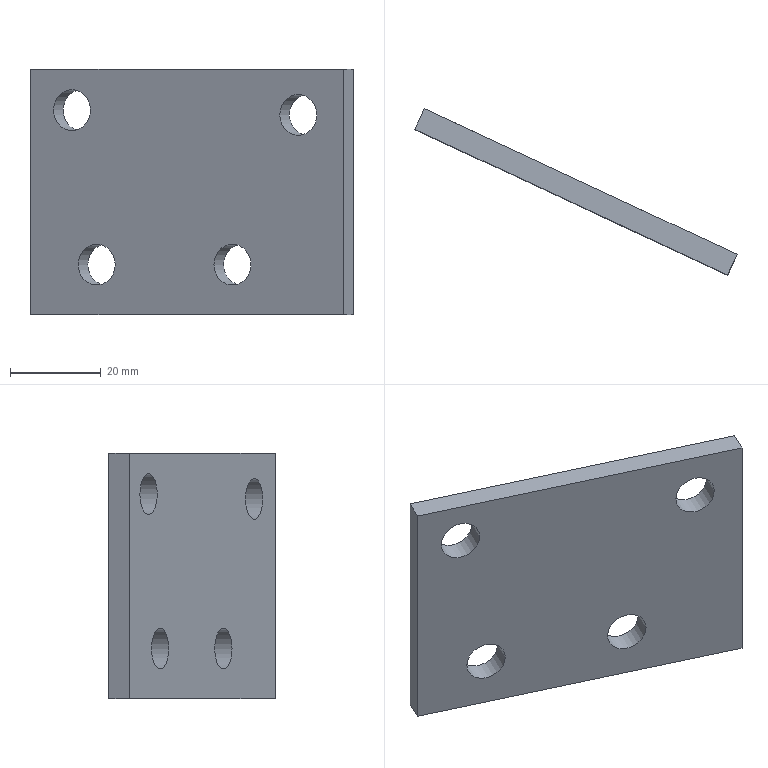Part | STEP file | gslz 2016.10.28-13_id86_x_t | 1 solid | 10 faces | box 70.992 x 36.651 x 54 mm | volume 19248 mm3 | plane 6 | cylinder 4 | commonest cylinder face diameters 9 x4
STEP:
#1=CARTESIAN_POINT('',(0.,0.,0.));
#2=DIRECTION('',(0.,0.,1.));
#3=DIRECTION('',(1.,0.,0.));
#4=AXIS2_PLACEMENT_3D('',#1,#2,#3);
#5=CARTESIAN_POINT('',(830.545,-269.865,-47.));
#6=VERTEX_POINT('',#5);
#7=CARTESIAN_POINT('',(826.467,-267.963,-47.));
#8=DIRECTION('',(-0.4226,-0.9063,0.));
#9=DIRECTION('',(0.9063,-0.4226,0.));
#10=AXIS2_PLACEMENT_3D('',#7,#8,#9);
#11=CIRCLE('',#10,4.5);
#12=CARTESIAN_POINT('',(835.05,-271.966,-72.139));
#13=DIRECTION('',(-0.4226,-0.9063,0.));
#14=DIRECTION('',(0.9063,-0.4226,0.));
#15=AXIS2_PLACEMENT_3D('',#12,#13,#14);
#16=PLANE('',#15);
#17=CARTESIAN_POINT('',(-9.471,25.139));
#18=DIRECTION('',(1.,0.));
#19=AXIS2_PLACEMENT_2D('',#17,#18);
#20=CIRCLE('',#19,4.5);
#21=(GEOMETRIC_REPRESENTATION_CONTEXT(2)PARAMETRIC_REPRESENTATION_CONTEXT()REPRESENTATION_CONTEXT('',''));
#22=DEFINITIONAL_REPRESENTATION('',(#20),#21);
#23=PCURVE('',#16,#22);
#24=CARTESIAN_POINT('',(826.467,-267.963,-47.));
#25=DIRECTION('',(-0.4226,-0.9063,0.));
#26=DIRECTION('',(0.9063,-0.4226,0.));
#27=AXIS2_PLACEMENT_3D('',#24,#25,#26);
#28=CYLINDRICAL_SURFACE('',#27,4.5);
#29=CARTESIAN_POINT('',(0.,-0.000007199));
#30=DIRECTION('',(1.,0.));
#31=VECTOR('',#30,1.);
#32=LINE('',#29,#31);
#33=(GEOMETRIC_REPRESENTATION_CONTEXT(2)PARAMETRIC_REPRESENTATION_CONTEXT()REPRESENTATION_CONTEXT('',''));
#34=DEFINITIONAL_REPRESENTATION('',(#32),#33);
#35=PCURVE('',#28,#34);
#36=SURFACE_CURVE('',#11,(#23,#35),.PCURVE_S1.);
#37=EDGE_CURVE('',#6,#6,#36,.T.);
#38=ORIENTED_EDGE('',*,*,#37,.T.);
#39=EDGE_LOOP('',(#38));
#40=FACE_BOUND('',#39,.T.);
#41=CARTESIAN_POINT('',(874.954,-290.573,-14.));
#42=VERTEX_POINT('',#41);
#43=CARTESIAN_POINT('',(870.876,-288.672,-14.));
#44=DIRECTION('',(-0.4226,-0.9063,0.));
#45=DIRECTION('',(0.9063,-0.4226,0.));
#46=AXIS2_PLACEMENT_3D('',#43,#44,#45);
#47=CIRCLE('',#46,4.5);
#48=CARTESIAN_POINT('',(39.529,58.139));
#49=DIRECTION('',(1.,0.));
#50=AXIS2_PLACEMENT_2D('',#48,#49);
#51=CIRCLE('',#50,4.5);
#52=(GEOMETRIC_REPRESENTATION_CONTEXT(2)PARAMETRIC_REPRESENTATION_CONTEXT()REPRESENTATION_CONTEXT('',''));
#53=DEFINITIONAL_REPRESENTATION('',(#51),#52);
#54=PCURVE('',#16,#53);
#55=CARTESIAN_POINT('',(870.876,-288.672,-14.));
#56=DIRECTION('',(-0.4226,-0.9063,0.));
#57=DIRECTION('',(0.9063,-0.4226,0.));
#58=AXIS2_PLACEMENT_3D('',#55,#56,#57);
#59=CYLINDRICAL_SURFACE('',#58,4.5);
#60=CARTESIAN_POINT('',(0.,0.000008835));
#61=DIRECTION('',(1.,0.));
#62=VECTOR('',#61,1.);
#63=LINE('',#60,#62);
#64=(GEOMETRIC_REPRESENTATION_CONTEXT(2)PARAMETRIC_REPRESENTATION_CONTEXT()REPRESENTATION_CONTEXT('',''));
#65=DEFINITIONAL_REPRESENTATION('',(#63),#64);
#66=PCURVE('',#59,#65);
#67=SURFACE_CURVE('',#47,(#54,#66),.PCURVE_S1.);
#68=EDGE_CURVE('',#42,#42,#67,.T.);
#69=ORIENTED_EDGE('',*,*,#68,.T.);
#70=EDGE_LOOP('',(#69));
#71=FACE_BOUND('',#70,.T.);
#72=CARTESIAN_POINT('',(860.453,-283.812,-47.));
#73=VERTEX_POINT('',#72);
#74=CARTESIAN_POINT('',(856.375,-281.91,-47.));
#75=DIRECTION('',(-0.4226,-0.9063,0.));
#76=DIRECTION('',(0.9063,-0.4226,0.));
#77=AXIS2_PLACEMENT_3D('',#74,#75,#76);
#78=CIRCLE('',#77,4.5);
#79=CARTESIAN_POINT('',(23.529,25.139));
#80=DIRECTION('',(1.,0.));
#81=AXIS2_PLACEMENT_2D('',#79,#80);
#82=CIRCLE('',#81,4.5);
#83=(GEOMETRIC_REPRESENTATION_CONTEXT(2)PARAMETRIC_REPRESENTATION_CONTEXT()REPRESENTATION_CONTEXT('',''));
#84=DEFINITIONAL_REPRESENTATION('',(#82),#83);
#85=PCURVE('',#16,#84);
#86=CARTESIAN_POINT('',(856.375,-281.91,-47.));
#87=DIRECTION('',(-0.4226,-0.9063,0.));
#88=DIRECTION('',(0.9063,-0.4226,0.));
#89=AXIS2_PLACEMENT_3D('',#86,#87,#88);
#90=CYLINDRICAL_SURFACE('',#89,4.5);
#91=CARTESIAN_POINT('',(0.,0.000007526));
#92=DIRECTION('',(1.,0.));
#93=VECTOR('',#92,1.);
#94=LINE('',#91,#93);
#95=(GEOMETRIC_REPRESENTATION_CONTEXT(2)PARAMETRIC_REPRESENTATION_CONTEXT()REPRESENTATION_CONTEXT('',''));
#96=DEFINITIONAL_REPRESENTATION('',(#94),#95);
#97=PCURVE('',#90,#96);
#98=SURFACE_CURVE('',#78,(#85,#97),.PCURVE_S1.);
#99=EDGE_CURVE('',#73,#73,#98,.T.);
#100=ORIENTED_EDGE('',*,*,#99,.F.);
#101=EDGE_LOOP('',(#100));
#102=FACE_BOUND('',#101,.F.);
#103=CARTESIAN_POINT('',(825.107,-267.329,-13.));
#104=VERTEX_POINT('',#103);
#105=CARTESIAN_POINT('',(821.029,-265.428,-13.));
#106=DIRECTION('',(-0.4226,-0.9063,0.));
#107=DIRECTION('',(0.9063,-0.4226,0.));
#108=AXIS2_PLACEMENT_3D('',#105,#106,#107);
#109=CIRCLE('',#108,4.5);
#110=CARTESIAN_POINT('',(-15.471,59.139));
#111=DIRECTION('',(1.,0.));
#112=AXIS2_PLACEMENT_2D('',#110,#111);
#113=CIRCLE('',#112,4.5);
#114=(GEOMETRIC_REPRESENTATION_CONTEXT(2)PARAMETRIC_REPRESENTATION_CONTEXT()REPRESENTATION_CONTEXT('',''));
#115=DEFINITIONAL_REPRESENTATION('',(#113),#114);
#116=PCURVE('',#16,#115);
#117=CARTESIAN_POINT('',(821.029,-265.428,-13.));
#118=DIRECTION('',(-0.4226,-0.9063,0.));
#119=DIRECTION('',(0.9063,-0.4226,0.));
#120=AXIS2_PLACEMENT_3D('',#117,#118,#119);
#121=CYLINDRICAL_SURFACE('',#120,4.5);
#122=CARTESIAN_POINT('',(0.,-0.000009162));
#123=DIRECTION('',(1.,0.));
#124=VECTOR('',#123,1.);
#125=LINE('',#122,#124);
#126=(GEOMETRIC_REPRESENTATION_CONTEXT(2)PARAMETRIC_REPRESENTATION_CONTEXT()REPRESENTATION_CONTEXT('',''));
#127=DEFINITIONAL_REPRESENTATION('',(#125),#126);
#128=PCURVE('',#121,#127);
#129=SURFACE_CURVE('',#109,(#116,#128),.PCURVE_S1.);
#130=EDGE_CURVE('',#104,#104,#129,.T.);
#131=ORIENTED_EDGE('',*,*,#130,.T.);
#132=EDGE_LOOP('',(#131));
#133=FACE_BOUND('',#132,.T.);
#134=CARTESIAN_POINT('',(880.845,-293.32,-58.));
#135=VERTEX_POINT('',#134);
#136=CARTESIAN_POINT('',(880.845,-293.32,-4.));
#137=VERTEX_POINT('',#136);
#138=CARTESIAN_POINT('',(880.845,-293.32,-72.139));
#139=DIRECTION('',(0.,0.,1.));
#140=VECTOR('',#139,1.);
#141=LINE('',#138,#140);
#142=CARTESIAN_POINT('',(50.529,0.));
#143=DIRECTION('',(0.,1.));
#144=VECTOR('',#143,1.);
#145=LINE('',#142,#144);
#146=(GEOMETRIC_REPRESENTATION_CONTEXT(2)PARAMETRIC_REPRESENTATION_CONTEXT()REPRESENTATION_CONTEXT('',''));
#147=DEFINITIONAL_REPRESENTATION('',(#145),#146);
#148=PCURVE('',#16,#147);
#149=CARTESIAN_POINT('',(858.446,-341.355,-72.139));
#150=DIRECTION('',(-0.9063,0.4226,0.));
#151=DIRECTION('',(-0.4226,-0.9063,0.));
#152=AXIS2_PLACEMENT_3D('',#149,#150,#151);
#153=PLANE('',#152);
#154=CARTESIAN_POINT('',(-53.,0.));
#155=DIRECTION('',(0.,1.));
#156=VECTOR('',#155,1.);
#157=LINE('',#154,#156);
#158=(GEOMETRIC_REPRESENTATION_CONTEXT(2)PARAMETRIC_REPRESENTATION_CONTEXT()REPRESENTATION_CONTEXT('',''));
#159=DEFINITIONAL_REPRESENTATION('',(#157),#158);
#160=PCURVE('',#153,#159);
#161=SURFACE_CURVE('',#141,(#148,#160),.PCURVE_S1.);
#162=EDGE_CURVE('',#135,#137,#161,.T.);
#163=ORIENTED_EDGE('',*,*,#162,.F.);
#164=CARTESIAN_POINT('',(811.966,-261.202,-58.));
#165=VERTEX_POINT('',#164);
#166=CARTESIAN_POINT('',(835.05,-271.966,-58.));
#167=DIRECTION('',(-0.9063,0.4226,0.));
#168=VECTOR('',#167,1.);
#169=LINE('',#166,#168);
#170=CARTESIAN_POINT('',(0.,14.139));
#171=DIRECTION('',(-1.,0.));
#172=VECTOR('',#171,1.);
#173=LINE('',#170,#172);
#174=(GEOMETRIC_REPRESENTATION_CONTEXT(2)PARAMETRIC_REPRESENTATION_CONTEXT()REPRESENTATION_CONTEXT('',''));
#175=DEFINITIONAL_REPRESENTATION('',(#173),#174);
#176=PCURVE('',#16,#175);
#177=CARTESIAN_POINT('',(-1525.071,939.124,-58.));
#178=DIRECTION('',(0.,0.,-1.));
#179=DIRECTION('',(-1.,0.,0.));
#180=AXIS2_PLACEMENT_3D('',#177,#178,#179);
#181=PLANE('',#180);
#182=CARTESIAN_POINT('',(-2360.122,-1211.09));
#183=DIRECTION('',(0.9063,0.4226));
#184=VECTOR('',#183,1.);
#185=LINE('',#182,#184);
#186=(GEOMETRIC_REPRESENTATION_CONTEXT(2)PARAMETRIC_REPRESENTATION_CONTEXT()REPRESENTATION_CONTEXT('',''));
#187=DEFINITIONAL_REPRESENTATION('',(#185),#186);
#188=PCURVE('',#181,#187);
#189=SURFACE_CURVE('',#169,(#176,#188),.PCURVE_S1.);
#190=EDGE_CURVE('',#135,#165,#189,.T.);
#191=ORIENTED_EDGE('',*,*,#190,.T.);
#192=CARTESIAN_POINT('',(811.966,-261.202,-4.));
#193=VERTEX_POINT('',#192);
#194=CARTESIAN_POINT('',(811.966,-261.202,-72.139));
#195=DIRECTION('',(0.,0.,1.));
#196=VECTOR('',#195,1.);
#197=LINE('',#194,#196);
#198=CARTESIAN_POINT('',(-25.471,0.));
#199=DIRECTION('',(0.,1.));
#200=VECTOR('',#199,1.);
#201=LINE('',#198,#200);
#202=(GEOMETRIC_REPRESENTATION_CONTEXT(2)PARAMETRIC_REPRESENTATION_CONTEXT()REPRESENTATION_CONTEXT('',''));
#203=DEFINITIONAL_REPRESENTATION('',(#201),#202);
#204=PCURVE('',#16,#203);
#205=CARTESIAN_POINT('',(789.567,-309.236,-72.139));
#206=DIRECTION('',(-0.9063,0.4226,0.));
#207=DIRECTION('',(-0.4226,-0.9063,0.));
#208=AXIS2_PLACEMENT_3D('',#205,#206,#207);
#209=PLANE('',#208);
#210=CARTESIAN_POINT('',(-53.,0.));
#211=DIRECTION('',(0.,1.));
#212=VECTOR('',#211,1.);
#213=LINE('',#210,#212);
#214=(GEOMETRIC_REPRESENTATION_CONTEXT(2)PARAMETRIC_REPRESENTATION_CONTEXT()REPRESENTATION_CONTEXT('',''));
#215=DEFINITIONAL_REPRESENTATION('',(#213),#214);
#216=PCURVE('',#209,#215);
#217=SURFACE_CURVE('',#197,(#204,#216),.PCURVE_S1.);
#218=EDGE_CURVE('',#165,#193,#217,.T.);
#219=ORIENTED_EDGE('',*,*,#218,.T.);
#220=CARTESIAN_POINT('',(835.05,-271.966,-4.));
#221=DIRECTION('',(-0.9063,0.4226,0.));
#222=VECTOR('',#221,1.);
#223=LINE('',#220,#222);
#224=CARTESIAN_POINT('',(0.,68.139));
#225=DIRECTION('',(-1.,0.));
#226=VECTOR('',#225,1.);
#227=LINE('',#224,#226);
#228=(GEOMETRIC_REPRESENTATION_CONTEXT(2)PARAMETRIC_REPRESENTATION_CONTEXT()REPRESENTATION_CONTEXT('',''));
#229=DEFINITIONAL_REPRESENTATION('',(#227),#228);
#230=PCURVE('',#16,#229);
#231=CARTESIAN_POINT('',(812.652,-320.,-4.));
#232=DIRECTION('',(0.,0.,-1.));
#233=DIRECTION('',(0.9397,0.342,0.));
#234=AXIS2_PLACEMENT_3D('',#231,#232,#233);
#235=PLANE('',#234);
#236=CARTESIAN_POINT('',(37.477,-37.477));
#237=DIRECTION('',(-0.7071,-0.7071));
#238=VECTOR('',#237,1.);
#239=LINE('',#236,#238);
#240=(GEOMETRIC_REPRESENTATION_CONTEXT(2)PARAMETRIC_REPRESENTATION_CONTEXT()REPRESENTATION_CONTEXT('',''));
#241=DEFINITIONAL_REPRESENTATION('',(#239),#240);
#242=PCURVE('',#235,#241);
#243=SURFACE_CURVE('',#223,(#230,#242),.PCURVE_S1.);
#244=EDGE_CURVE('',#137,#193,#243,.T.);
#245=ORIENTED_EDGE('',*,*,#244,.F.);
#246=EDGE_LOOP('',(#163,#191,#219,#245));
#247=FACE_BOUND('',#246,.T.);
#248=ADVANCED_FACE('',(#40,#71,#102,#133,#247),#16,.F.);
#249=CARTESIAN_POINT('',(878.732,-297.852,-4.));
#250=VERTEX_POINT('',#249);
#251=CARTESIAN_POINT('',(858.446,-341.355,-4.));
#252=DIRECTION('',(0.4226,0.9063,0.));
#253=VECTOR('',#252,1.);
#254=LINE('',#251,#253);
#255=CARTESIAN_POINT('',(0.,68.139));
#256=DIRECTION('',(-1.,0.));
#257=VECTOR('',#256,1.);
#258=LINE('',#255,#257);
#259=(GEOMETRIC_REPRESENTATION_CONTEXT(2)PARAMETRIC_REPRESENTATION_CONTEXT()REPRESENTATION_CONTEXT('',''));
#260=DEFINITIONAL_REPRESENTATION('',(#258),#259);
#261=PCURVE('',#153,#260);
#262=CARTESIAN_POINT('',(35.729,35.729));
#263=DIRECTION('',(0.7071,-0.7071));
#264=VECTOR('',#263,1.);
#265=LINE('',#262,#264);
#266=(GEOMETRIC_REPRESENTATION_CONTEXT(2)PARAMETRIC_REPRESENTATION_CONTEXT()REPRESENTATION_CONTEXT('',''));
#267=DEFINITIONAL_REPRESENTATION('',(#265),#266);
#268=PCURVE('',#235,#267);
#269=SURFACE_CURVE('',#254,(#261,#268),.PCURVE_S1.);
#270=EDGE_CURVE('',#250,#137,#269,.T.);
#271=ORIENTED_EDGE('',*,*,#270,.F.);
#272=CARTESIAN_POINT('',(878.732,-297.852,-58.));
#273=VERTEX_POINT('',#272);
#274=CARTESIAN_POINT('',(878.732,-297.852,-72.139));
#275=DIRECTION('',(0.,0.,-1.));
#276=VECTOR('',#275,1.);
#277=LINE('',#274,#276);
#278=CARTESIAN_POINT('',(-48.,0.));
#279=DIRECTION('',(0.,-1.));
#280=VECTOR('',#279,1.);
#281=LINE('',#278,#280);
#282=(GEOMETRIC_REPRESENTATION_CONTEXT(2)PARAMETRIC_REPRESENTATION_CONTEXT()REPRESENTATION_CONTEXT('',''));
#283=DEFINITIONAL_REPRESENTATION('',(#281),#282);
#284=PCURVE('',#153,#283);
#285=CARTESIAN_POINT('',(844.292,-281.793,-33.75));
#286=DIRECTION('',(0.4226,0.9063,0.));
#287=DIRECTION('',(-0.9063,0.4226,0.));
#288=AXIS2_PLACEMENT_3D('',#285,#286,#287);
#289=PLANE('',#288);
#290=CARTESIAN_POINT('',(-38.,-38.389));
#291=DIRECTION('',(0.,-1.));
#292=VECTOR('',#291,1.);
#293=LINE('',#290,#292);
#294=(GEOMETRIC_REPRESENTATION_CONTEXT(2)PARAMETRIC_REPRESENTATION_CONTEXT()REPRESENTATION_CONTEXT('',''));
#295=DEFINITIONAL_REPRESENTATION('',(#293),#294);
#296=PCURVE('',#289,#295);
#297=SURFACE_CURVE('',#277,(#284,#296),.PCURVE_S1.);
#298=EDGE_CURVE('',#250,#273,#297,.T.);
#299=ORIENTED_EDGE('',*,*,#298,.T.);
#300=CARTESIAN_POINT('',(923.187,-202.518,-58.));
#301=DIRECTION('',(-0.4226,-0.9063,0.));
#302=VECTOR('',#301,1.);
#303=LINE('',#300,#302);
#304=CARTESIAN_POINT('',(-153.19,14.139));
#305=DIRECTION('',(1.,0.));
#306=VECTOR('',#305,1.);
#307=LINE('',#304,#306);
#308=(GEOMETRIC_REPRESENTATION_CONTEXT(2)PARAMETRIC_REPRESENTATION_CONTEXT()REPRESENTATION_CONTEXT('',''));
#309=DEFINITIONAL_REPRESENTATION('',(#307),#308);
#310=PCURVE('',#153,#309);
#311=CARTESIAN_POINT('',(-2448.259,-1141.642));
#312=DIRECTION('',(0.4226,-0.9063));
#313=VECTOR('',#312,1.);
#314=LINE('',#311,#313);
#315=(GEOMETRIC_REPRESENTATION_CONTEXT(2)PARAMETRIC_REPRESENTATION_CONTEXT()REPRESENTATION_CONTEXT('',''));
#316=DEFINITIONAL_REPRESENTATION('',(#314),#315);
#317=PCURVE('',#181,#316);
#318=SURFACE_CURVE('',#303,(#310,#317),.PCURVE_S1.);
#319=EDGE_CURVE('',#135,#273,#318,.T.);
#320=ORIENTED_EDGE('',*,*,#319,.F.);
#321=ORIENTED_EDGE('',*,*,#162,.T.);
#322=EDGE_LOOP('',(#271,#299,#320,#321));
#323=FACE_BOUND('',#322,.T.);
#324=ADVANCED_FACE('',(#323),#153,.F.);
#325=CARTESIAN_POINT('',(809.853,-265.733,-4.));
#326=VERTEX_POINT('',#325);
#327=CARTESIAN_POINT('',(789.567,-309.236,-4.));
#328=DIRECTION('',(0.4226,0.9063,0.));
#329=VECTOR('',#328,1.);
#330=LINE('',#327,#329);
#331=CARTESIAN_POINT('',(-18.011,-18.011));
#332=DIRECTION('',(0.7071,-0.7071));
#333=VECTOR('',#332,1.);
#334=LINE('',#331,#333);
#335=(GEOMETRIC_REPRESENTATION_CONTEXT(2)PARAMETRIC_REPRESENTATION_CONTEXT()REPRESENTATION_CONTEXT('',''));
#336=DEFINITIONAL_REPRESENTATION('',(#334),#335);
#337=PCURVE('',#235,#336);
#338=CARTESIAN_POINT('',(0.,68.139));
#339=DIRECTION('',(-1.,0.));
#340=VECTOR('',#339,1.);
#341=LINE('',#338,#340);
#342=(GEOMETRIC_REPRESENTATION_CONTEXT(2)PARAMETRIC_REPRESENTATION_CONTEXT()REPRESENTATION_CONTEXT('',''));
#343=DEFINITIONAL_REPRESENTATION('',(#341),#342);
#344=PCURVE('',#209,#343);
#345=SURFACE_CURVE('',#330,(#337,#344),.PCURVE_S1.);
#346=EDGE_CURVE('',#326,#193,#345,.T.);
#347=ORIENTED_EDGE('',*,*,#346,.F.);
#348=CARTESIAN_POINT('',(832.937,-276.498,-4.));
#349=DIRECTION('',(0.9063,-0.4226,0.));
#350=VECTOR('',#349,1.);
#351=LINE('',#348,#350);
#352=CARTESIAN_POINT('',(33.941,-33.941));
#353=DIRECTION('',(0.7071,0.7071));
#354=VECTOR('',#353,1.);
#355=LINE('',#352,#354);
#356=(GEOMETRIC_REPRESENTATION_CONTEXT(2)PARAMETRIC_REPRESENTATION_CONTEXT()REPRESENTATION_CONTEXT('',''));
#357=DEFINITIONAL_REPRESENTATION('',(#355),#356);
#358=PCURVE('',#235,#357);
#359=CARTESIAN_POINT('',(12.529,29.75));
#360=DIRECTION('',(-1.,0.));
#361=VECTOR('',#360,1.);
#362=LINE('',#359,#361);
#363=(GEOMETRIC_REPRESENTATION_CONTEXT(2)PARAMETRIC_REPRESENTATION_CONTEXT()REPRESENTATION_CONTEXT('',''));
#364=DEFINITIONAL_REPRESENTATION('',(#362),#363);
#365=PCURVE('',#289,#364);
#366=SURFACE_CURVE('',#351,(#358,#365),.PCURVE_S1.);
#367=EDGE_CURVE('',#326,#250,#366,.T.);
#368=ORIENTED_EDGE('',*,*,#367,.T.);
#369=ORIENTED_EDGE('',*,*,#270,.T.);
#370=ORIENTED_EDGE('',*,*,#244,.T.);
#371=EDGE_LOOP('',(#347,#368,#369,#370));
#372=FACE_BOUND('',#371,.T.);
#373=ADVANCED_FACE('',(#372),#235,.F.);
#374=CARTESIAN_POINT('',(809.853,-265.733,-58.));
#375=VERTEX_POINT('',#374);
#376=CARTESIAN_POINT('',(809.853,-265.733,-33.75));
#377=DIRECTION('',(0.,0.,1.));
#378=VECTOR('',#377,1.);
#379=LINE('',#376,#378);
#380=CARTESIAN_POINT('',(-48.,38.389));
#381=DIRECTION('',(0.,1.));
#382=VECTOR('',#381,1.);
#383=LINE('',#380,#382);
#384=(GEOMETRIC_REPRESENTATION_CONTEXT(2)PARAMETRIC_REPRESENTATION_CONTEXT()REPRESENTATION_CONTEXT('',''));
#385=DEFINITIONAL_REPRESENTATION('',(#383),#384);
#386=PCURVE('',#209,#385);
#387=CARTESIAN_POINT('',(38.,0.));
#388=DIRECTION('',(0.,1.));
#389=VECTOR('',#388,1.);
#390=LINE('',#387,#389);
#391=(GEOMETRIC_REPRESENTATION_CONTEXT(2)PARAMETRIC_REPRESENTATION_CONTEXT()REPRESENTATION_CONTEXT('',''));
#392=DEFINITIONAL_REPRESENTATION('',(#390),#391);
#393=PCURVE('',#289,#392);
#394=SURFACE_CURVE('',#379,(#386,#393),.PCURVE_S1.);
#395=EDGE_CURVE('',#375,#326,#394,.T.);
#396=ORIENTED_EDGE('',*,*,#395,.T.);
#397=ORIENTED_EDGE('',*,*,#346,.T.);
#398=ORIENTED_EDGE('',*,*,#218,.F.);
#399=CARTESIAN_POINT('',(789.567,-309.236,-58.));
#400=DIRECTION('',(0.4226,0.9063,0.));
#401=VECTOR('',#400,1.);
#402=LINE('',#399,#401);
#403=CARTESIAN_POINT('',(0.,14.139));
#404=DIRECTION('',(-1.,0.));
#405=VECTOR('',#404,1.);
#406=LINE('',#403,#405);
#407=(GEOMETRIC_REPRESENTATION_CONTEXT(2)PARAMETRIC_REPRESENTATION_CONTEXT()REPRESENTATION_CONTEXT('',''));
#408=DEFINITIONAL_REPRESENTATION('',(#406),#407);
#409=PCURVE('',#209,#408);
#410=CARTESIAN_POINT('',(-2314.638,-1248.36));
#411=DIRECTION('',(-0.4226,0.9063));
#412=VECTOR('',#411,1.);
#413=LINE('',#410,#412);
#414=(GEOMETRIC_REPRESENTATION_CONTEXT(2)PARAMETRIC_REPRESENTATION_CONTEXT()REPRESENTATION_CONTEXT('',''));
#415=DEFINITIONAL_REPRESENTATION('',(#413),#414);
#416=PCURVE('',#181,#415);
#417=SURFACE_CURVE('',#402,(#409,#416),.PCURVE_S1.);
#418=EDGE_CURVE('',#375,#165,#417,.T.);
#419=ORIENTED_EDGE('',*,*,#418,.F.);
#420=EDGE_LOOP('',(#396,#397,#398,#419));
#421=FACE_BOUND('',#420,.T.);
#422=ADVANCED_FACE('',(#421),#209,.T.);
#423=CARTESIAN_POINT('',(814.837,-268.057,-13.));
#424=VERTEX_POINT('',#423);
#425=CARTESIAN_POINT('',(822.994,-271.861,-13.));
#426=VERTEX_POINT('',#425);
#427=CARTESIAN_POINT('',(818.916,-269.959,-13.));
#428=DIRECTION('',(0.4226,0.9063,0.));
#429=DIRECTION('',(-0.9063,0.4226,0.));
#430=AXIS2_PLACEMENT_3D('',#427,#428,#429);
#431=CIRCLE('',#430,4.5);
#432=CARTESIAN_POINT('',(3.142,5.));
#433=DIRECTION('',(-1.,0.));
#434=VECTOR('',#433,1.);
#435=LINE('',#432,#434);
#436=(GEOMETRIC_REPRESENTATION_CONTEXT(2)PARAMETRIC_REPRESENTATION_CONTEXT()REPRESENTATION_CONTEXT('',''));
#437=DEFINITIONAL_REPRESENTATION('',(#435),#436);
#438=PCURVE('',#121,#437);
#439=CARTESIAN_POINT('',(28.,20.75));
#440=DIRECTION('',(1.,0.));
#441=AXIS2_PLACEMENT_2D('',#439,#440);
#442=CIRCLE('',#441,4.5);
#443=(GEOMETRIC_REPRESENTATION_CONTEXT(2)PARAMETRIC_REPRESENTATION_CONTEXT()REPRESENTATION_CONTEXT('',''));
#444=DEFINITIONAL_REPRESENTATION('',(#442),#443);
#445=PCURVE('',#289,#444);
#446=SURFACE_CURVE('',#431,(#438,#445),.PCURVE_S1.);
#447=EDGE_CURVE('',#424,#426,#446,.T.);
#448=ORIENTED_EDGE('',*,*,#447,.T.);
#449=CARTESIAN_POINT('',(825.107,-267.329,-13.));
#450=CARTESIAN_POINT('',(822.994,-271.861,-13.));
#451=B_SPLINE_CURVE_WITH_KNOTS('',1,(#449,#450),.UNSPECIFIED.,.F.,.F.,(2,2),(-0.000009162,5.),.PIECEWISE_BEZIER_KNOTS.);
#452=CARTESIAN_POINT('',(0.,0.));
#453=DIRECTION('',(0.,1.));
#454=VECTOR('',#453,1.);
#455=LINE('',#452,#454);
#456=(GEOMETRIC_REPRESENTATION_CONTEXT(2)PARAMETRIC_REPRESENTATION_CONTEXT()REPRESENTATION_CONTEXT('',''));
#457=DEFINITIONAL_REPRESENTATION('',(#455),#456);
#458=PCURVE('',#121,#457);
#459=CARTESIAN_POINT('',(6.283,0.));
#460=DIRECTION('',(0.,1.));
#461=VECTOR('',#460,1.);
#462=LINE('',#459,#461);
#463=(GEOMETRIC_REPRESENTATION_CONTEXT(2)PARAMETRIC_REPRESENTATION_CONTEXT()REPRESENTATION_CONTEXT('',''));
#464=DEFINITIONAL_REPRESENTATION('',(#462),#463);
#465=PCURVE('',#121,#464);
#466=SEAM_CURVE('',#451,(#458,#465),.PCURVE_S1.);
#467=EDGE_CURVE('',#104,#426,#466,.T.);
#468=ORIENTED_EDGE('',*,*,#467,.F.);
#469=ORIENTED_EDGE('',*,*,#130,.T.);
#470=ORIENTED_EDGE('',*,*,#467,.T.);
#471=CARTESIAN_POINT('',(818.916,-269.959,-13.));
#472=DIRECTION('',(0.4226,0.9063,0.));
#473=DIRECTION('',(-0.9063,0.4226,0.));
#474=AXIS2_PLACEMENT_3D('',#471,#472,#473);
#475=CIRCLE('',#474,4.5);
#476=CARTESIAN_POINT('',(9.425,5.));
#477=DIRECTION('',(-1.,0.));
#478=VECTOR('',#477,1.);
#479=LINE('',#476,#478);
#480=(GEOMETRIC_REPRESENTATION_CONTEXT(2)PARAMETRIC_REPRESENTATION_CONTEXT()REPRESENTATION_CONTEXT('',''));
#481=DEFINITIONAL_REPRESENTATION('',(#479),#480);
#482=PCURVE('',#121,#481);
#483=CARTESIAN_POINT('',(28.,20.75));
#484=DIRECTION('',(1.,0.));
#485=AXIS2_PLACEMENT_2D('',#483,#484);
#486=CIRCLE('',#485,4.5);
#487=(GEOMETRIC_REPRESENTATION_CONTEXT(2)PARAMETRIC_REPRESENTATION_CONTEXT()REPRESENTATION_CONTEXT('',''));
#488=DEFINITIONAL_REPRESENTATION('',(#486),#487);
#489=PCURVE('',#289,#488);
#490=SURFACE_CURVE('',#475,(#482,#489),.PCURVE_S1.);
#491=EDGE_CURVE('',#426,#424,#490,.T.);
#492=ORIENTED_EDGE('',*,*,#491,.T.);
#493=EDGE_LOOP('',(#448,#468,#469,#470,#492));
#494=FACE_BOUND('',#493,.F.);
#495=ADVANCED_FACE('',(#494),#121,.F.);
#496=CARTESIAN_POINT('',(850.183,-284.54,-47.));
#497=VERTEX_POINT('',#496);
#498=CARTESIAN_POINT('',(858.34,-288.343,-47.));
#499=VERTEX_POINT('',#498);
#500=CARTESIAN_POINT('',(854.262,-286.441,-47.));
#501=DIRECTION('',(0.4226,0.9063,0.));
#502=DIRECTION('',(-0.9063,0.4226,0.));
#503=AXIS2_PLACEMENT_3D('',#500,#501,#502);
#504=CIRCLE('',#503,4.5);
#505=CARTESIAN_POINT('',(3.142,5.));
#506=DIRECTION('',(-1.,0.));
#507=VECTOR('',#506,1.);
#508=LINE('',#505,#507);
#509=(GEOMETRIC_REPRESENTATION_CONTEXT(2)PARAMETRIC_REPRESENTATION_CONTEXT()REPRESENTATION_CONTEXT('',''));
#510=DEFINITIONAL_REPRESENTATION('',(#508),#509);
#511=PCURVE('',#90,#510);
#512=CARTESIAN_POINT('',(-11.,-13.25));
#513=DIRECTION('',(1.,0.));
#514=AXIS2_PLACEMENT_2D('',#512,#513);
#515=CIRCLE('',#514,4.5);
#516=(GEOMETRIC_REPRESENTATION_CONTEXT(2)PARAMETRIC_REPRESENTATION_CONTEXT()REPRESENTATION_CONTEXT('',''));
#517=DEFINITIONAL_REPRESENTATION('',(#515),#516);
#518=PCURVE('',#289,#517);
#519=SURFACE_CURVE('',#504,(#511,#518),.PCURVE_S1.);
#520=EDGE_CURVE('',#497,#499,#519,.T.);
#521=ORIENTED_EDGE('',*,*,#520,.T.);
#522=CARTESIAN_POINT('',(860.453,-283.812,-47.));
#523=CARTESIAN_POINT('',(858.34,-288.343,-47.));
#524=B_SPLINE_CURVE_WITH_KNOTS('',1,(#522,#523),.UNSPECIFIED.,.F.,.F.,(2,2),(0.000007526,5.),.PIECEWISE_BEZIER_KNOTS.);
#525=CARTESIAN_POINT('',(0.,0.));
#526=DIRECTION('',(0.,1.));
#527=VECTOR('',#526,1.);
#528=LINE('',#525,#527);
#529=(GEOMETRIC_REPRESENTATION_CONTEXT(2)PARAMETRIC_REPRESENTATION_CONTEXT()REPRESENTATION_CONTEXT('',''));
#530=DEFINITIONAL_REPRESENTATION('',(#528),#529);
#531=PCURVE('',#90,#530);
#532=CARTESIAN_POINT('',(6.283,0.));
#533=DIRECTION('',(0.,1.));
#534=VECTOR('',#533,1.);
#535=LINE('',#532,#534);
#536=(GEOMETRIC_REPRESENTATION_CONTEXT(2)PARAMETRIC_REPRESENTATION_CONTEXT()REPRESENTATION_CONTEXT('',''));
#537=DEFINITIONAL_REPRESENTATION('',(#535),#536);
#538=PCURVE('',#90,#537);
#539=SEAM_CURVE('',#524,(#531,#538),.PCURVE_S1.);
#540=EDGE_CURVE('',#73,#499,#539,.T.);
#541=ORIENTED_EDGE('',*,*,#540,.F.);
#542=ORIENTED_EDGE('',*,*,#99,.T.);
#543=ORIENTED_EDGE('',*,*,#540,.T.);
#544=CARTESIAN_POINT('',(854.262,-286.441,-47.));
#545=DIRECTION('',(0.4226,0.9063,0.));
#546=DIRECTION('',(-0.9063,0.4226,0.));
#547=AXIS2_PLACEMENT_3D('',#544,#545,#546);
#548=CIRCLE('',#547,4.5);
#549=CARTESIAN_POINT('',(9.425,5.));
#550=DIRECTION('',(-1.,0.));
#551=VECTOR('',#550,1.);
#552=LINE('',#549,#551);
#553=(GEOMETRIC_REPRESENTATION_CONTEXT(2)PARAMETRIC_REPRESENTATION_CONTEXT()REPRESENTATION_CONTEXT('',''));
#554=DEFINITIONAL_REPRESENTATION('',(#552),#553);
#555=PCURVE('',#90,#554);
#556=CARTESIAN_POINT('',(-11.,-13.25));
#557=DIRECTION('',(1.,0.));
#558=AXIS2_PLACEMENT_2D('',#556,#557);
#559=CIRCLE('',#558,4.5);
#560=(GEOMETRIC_REPRESENTATION_CONTEXT(2)PARAMETRIC_REPRESENTATION_CONTEXT()REPRESENTATION_CONTEXT('',''));
#561=DEFINITIONAL_REPRESENTATION('',(#559),#560);
#562=PCURVE('',#289,#561);
#563=SURFACE_CURVE('',#548,(#555,#562),.PCURVE_S1.);
#564=EDGE_CURVE('',#499,#497,#563,.T.);
#565=ORIENTED_EDGE('',*,*,#564,.T.);
#566=EDGE_LOOP('',(#521,#541,#542,#543,#565));
#567=FACE_BOUND('',#566,.F.);
#568=ADVANCED_FACE('',(#567),#90,.F.);
#569=CARTESIAN_POINT('',(872.841,-295.105,-14.));
#570=VERTEX_POINT('',#569);
#571=CARTESIAN_POINT('',(864.684,-291.301,-14.));
#572=VERTEX_POINT('',#571);
#573=CARTESIAN_POINT('',(868.763,-293.203,-14.));
#574=DIRECTION('',(-0.4226,-0.9063,0.));
#575=DIRECTION('',(-0.9063,0.4226,0.));
#576=AXIS2_PLACEMENT_3D('',#573,#574,#575);
#577=CIRCLE('',#576,4.5);
#578=CARTESIAN_POINT('',(-3.142,5.));
#579=DIRECTION('',(1.,0.));
#580=VECTOR('',#579,1.);
#581=LINE('',#578,#580);
#582=(GEOMETRIC_REPRESENTATION_CONTEXT(2)PARAMETRIC_REPRESENTATION_CONTEXT()REPRESENTATION_CONTEXT('',''));
#583=DEFINITIONAL_REPRESENTATION('',(#581),#582);
#584=PCURVE('',#59,#583);
#585=CARTESIAN_POINT('',(-22.5,19.75));
#586=CARTESIAN_POINT('',(-22.5,11.956));
#587=CARTESIAN_POINT('',(-29.25,15.853));
#588=CARTESIAN_POINT('',(-36.,19.75));
#589=CARTESIAN_POINT('',(-29.25,23.647));
#590=CARTESIAN_POINT('',(-22.5,27.544));
#591=CARTESIAN_POINT('',(-22.5,19.75));
#592=(BOUNDED_CURVE()B_SPLINE_CURVE(2,(#585,#586,#587,#588,#589,#590,#591),.UNSPECIFIED.,.T.,.F.)B_SPLINE_CURVE_WITH_KNOTS((1,2,2,2,2,1),(-2.094,0.,2.094,4.189,6.283,8.378),.UNSPECIFIED.)CURVE()GEOMETRIC_REPRESENTATION_ITEM()RATIONAL_B_SPLINE_CURVE((1.,0.5,1.,0.5,1.,0.5,1.))REPRESENTATION_ITEM(''));
#593=(GEOMETRIC_REPRESENTATION_CONTEXT(2)PARAMETRIC_REPRESENTATION_CONTEXT()REPRESENTATION_CONTEXT('',''));
#594=DEFINITIONAL_REPRESENTATION('',(#592),#593);
#595=PCURVE('',#289,#594);
#596=SURFACE_CURVE('',#577,(#584,#595),.PCURVE_S1.);
#597=EDGE_CURVE('',#570,#572,#596,.T.);
#598=ORIENTED_EDGE('',*,*,#597,.F.);
#599=CARTESIAN_POINT('',(874.954,-290.573,-14.));
#600=CARTESIAN_POINT('',(872.841,-295.105,-14.));
#601=B_SPLINE_CURVE_WITH_KNOTS('',1,(#599,#600),.UNSPECIFIED.,.F.,.F.,(2,2),(0.000008835,5.),.PIECEWISE_BEZIER_KNOTS.);
#602=CARTESIAN_POINT('',(0.,0.));
#603=DIRECTION('',(0.,1.));
#604=VECTOR('',#603,1.);
#605=LINE('',#602,#604);
#606=(GEOMETRIC_REPRESENTATION_CONTEXT(2)PARAMETRIC_REPRESENTATION_CONTEXT()REPRESENTATION_CONTEXT('',''));
#607=DEFINITIONAL_REPRESENTATION('',(#605),#606);
#608=PCURVE('',#59,#607);
#609=CARTESIAN_POINT('',(6.283,0.));
#610=DIRECTION('',(0.,1.));
#611=VECTOR('',#610,1.);
#612=LINE('',#609,#611);
#613=(GEOMETRIC_REPRESENTATION_CONTEXT(2)PARAMETRIC_REPRESENTATION_CONTEXT()REPRESENTATION_CONTEXT('',''));
#614=DEFINITIONAL_REPRESENTATION('',(#612),#613);
#615=PCURVE('',#59,#614);
#616=SEAM_CURVE('',#601,(#608,#615),.PCURVE_S1.);
#617=EDGE_CURVE('',#42,#570,#616,.T.);
#618=ORIENTED_EDGE('',*,*,#617,.F.);
#619=ORIENTED_EDGE('',*,*,#68,.T.);
#620=ORIENTED_EDGE('',*,*,#617,.T.);
#621=CARTESIAN_POINT('',(868.763,-293.203,-14.));
#622=DIRECTION('',(-0.4226,-0.9063,0.));
#623=DIRECTION('',(-0.9063,0.4226,0.));
#624=AXIS2_PLACEMENT_3D('',#621,#622,#623);
#625=CIRCLE('',#624,4.5);
#626=CARTESIAN_POINT('',(3.142,5.));
#627=DIRECTION('',(1.,0.));
#628=VECTOR('',#627,1.);
#629=LINE('',#626,#628);
#630=(GEOMETRIC_REPRESENTATION_CONTEXT(2)PARAMETRIC_REPRESENTATION_CONTEXT()REPRESENTATION_CONTEXT('',''));
#631=DEFINITIONAL_REPRESENTATION('',(#629),#630);
#632=PCURVE('',#59,#631);
#633=CARTESIAN_POINT('',(-22.5,19.75));
#634=CARTESIAN_POINT('',(-22.5,11.956));
#635=CARTESIAN_POINT('',(-29.25,15.853));
#636=CARTESIAN_POINT('',(-36.,19.75));
#637=CARTESIAN_POINT('',(-29.25,23.647));
#638=CARTESIAN_POINT('',(-22.5,27.544));
#639=CARTESIAN_POINT('',(-22.5,19.75));
#640=(BOUNDED_CURVE()B_SPLINE_CURVE(2,(#633,#634,#635,#636,#637,#638,#639),.UNSPECIFIED.,.T.,.F.)B_SPLINE_CURVE_WITH_KNOTS((1,2,2,2,2,1),(-2.094,0.,2.094,4.189,6.283,8.378),.UNSPECIFIED.)CURVE()GEOMETRIC_REPRESENTATION_ITEM()RATIONAL_B_SPLINE_CURVE((1.,0.5,1.,0.5,1.,0.5,1.))REPRESENTATION_ITEM(''));
#641=(GEOMETRIC_REPRESENTATION_CONTEXT(2)PARAMETRIC_REPRESENTATION_CONTEXT()REPRESENTATION_CONTEXT('',''));
#642=DEFINITIONAL_REPRESENTATION('',(#640),#641);
#643=PCURVE('',#289,#642);
#644=SURFACE_CURVE('',#625,(#632,#643),.PCURVE_S1.);
#645=EDGE_CURVE('',#572,#570,#644,.T.);
#646=ORIENTED_EDGE('',*,*,#645,.F.);
#647=EDGE_LOOP('',(#598,#618,#619,#620,#646));
#648=FACE_BOUND('',#647,.F.);
#649=ADVANCED_FACE('',(#648),#59,.F.);
#650=CARTESIAN_POINT('',(828.432,-274.397,-47.));
#651=VERTEX_POINT('',#650);
#652=CARTESIAN_POINT('',(820.275,-270.593,-47.));
#653=VERTEX_POINT('',#652);
#654=CARTESIAN_POINT('',(824.354,-272.495,-47.));
#655=DIRECTION('',(-0.4226,-0.9063,0.));
#656=DIRECTION('',(-0.9063,0.4226,0.));
#657=AXIS2_PLACEMENT_3D('',#654,#655,#656);
#658=CIRCLE('',#657,4.5);
#659=CARTESIAN_POINT('',(-3.142,5.));
#660=DIRECTION('',(1.,0.));
#661=VECTOR('',#660,1.);
#662=LINE('',#659,#661);
#663=(GEOMETRIC_REPRESENTATION_CONTEXT(2)PARAMETRIC_REPRESENTATION_CONTEXT()REPRESENTATION_CONTEXT('',''));
#664=DEFINITIONAL_REPRESENTATION('',(#662),#663);
#665=PCURVE('',#28,#664);
#666=CARTESIAN_POINT('',(26.5,-13.25));
#667=CARTESIAN_POINT('',(26.5,-21.044));
#668=CARTESIAN_POINT('',(19.75,-17.147));
#669=CARTESIAN_POINT('',(13.,-13.25));
#670=CARTESIAN_POINT('',(19.75,-9.353));
#671=CARTESIAN_POINT('',(26.5,-5.456));
#672=CARTESIAN_POINT('',(26.5,-13.25));
#673=(BOUNDED_CURVE()B_SPLINE_CURVE(2,(#666,#667,#668,#669,#670,#671,#672),.UNSPECIFIED.,.T.,.F.)B_SPLINE_CURVE_WITH_KNOTS((1,2,2,2,2,1),(-2.094,0.,2.094,4.189,6.283,8.378),.UNSPECIFIED.)CURVE()GEOMETRIC_REPRESENTATION_ITEM()RATIONAL_B_SPLINE_CURVE((1.,0.5,1.,0.5,1.,0.5,1.))REPRESENTATION_ITEM(''));
#674=(GEOMETRIC_REPRESENTATION_CONTEXT(2)PARAMETRIC_REPRESENTATION_CONTEXT()REPRESENTATION_CONTEXT('',''));
#675=DEFINITIONAL_REPRESENTATION('',(#673),#674);
#676=PCURVE('',#289,#675);
#677=SURFACE_CURVE('',#658,(#665,#676),.PCURVE_S1.);
#678=EDGE_CURVE('',#651,#653,#677,.T.);
#679=ORIENTED_EDGE('',*,*,#678,.F.);
#680=CARTESIAN_POINT('',(830.545,-269.865,-47.));
#681=CARTESIAN_POINT('',(828.432,-274.397,-47.));
#682=B_SPLINE_CURVE_WITH_KNOTS('',1,(#680,#681),.UNSPECIFIED.,.F.,.F.,(2,2),(-0.000007199,5.),.PIECEWISE_BEZIER_KNOTS.);
#683=CARTESIAN_POINT('',(0.,0.));
#684=DIRECTION('',(0.,1.));
#685=VECTOR('',#684,1.);
#686=LINE('',#683,#685);
#687=(GEOMETRIC_REPRESENTATION_CONTEXT(2)PARAMETRIC_REPRESENTATION_CONTEXT()REPRESENTATION_CONTEXT('',''));
#688=DEFINITIONAL_REPRESENTATION('',(#686),#687);
#689=PCURVE('',#28,#688);
#690=CARTESIAN_POINT('',(6.283,0.));
#691=DIRECTION('',(0.,1.));
#692=VECTOR('',#691,1.);
#693=LINE('',#690,#692);
#694=(GEOMETRIC_REPRESENTATION_CONTEXT(2)PARAMETRIC_REPRESENTATION_CONTEXT()REPRESENTATION_CONTEXT('',''));
#695=DEFINITIONAL_REPRESENTATION('',(#693),#694);
#696=PCURVE('',#28,#695);
#697=SEAM_CURVE('',#682,(#689,#696),.PCURVE_S1.);
#698=EDGE_CURVE('',#6,#651,#697,.T.);
#699=ORIENTED_EDGE('',*,*,#698,.F.);
#700=ORIENTED_EDGE('',*,*,#37,.T.);
#701=ORIENTED_EDGE('',*,*,#698,.T.);
#702=CARTESIAN_POINT('',(824.354,-272.495,-47.));
#703=DIRECTION('',(-0.4226,-0.9063,0.));
#704=DIRECTION('',(-0.9063,0.4226,0.));
#705=AXIS2_PLACEMENT_3D('',#702,#703,#704);
#706=CIRCLE('',#705,4.5);
#707=CARTESIAN_POINT('',(3.142,5.));
#708=DIRECTION('',(1.,0.));
#709=VECTOR('',#708,1.);
#710=LINE('',#707,#709);
#711=(GEOMETRIC_REPRESENTATION_CONTEXT(2)PARAMETRIC_REPRESENTATION_CONTEXT()REPRESENTATION_CONTEXT('',''));
#712=DEFINITIONAL_REPRESENTATION('',(#710),#711);
#713=PCURVE('',#28,#712);
#714=CARTESIAN_POINT('',(26.5,-13.25));
#715=CARTESIAN_POINT('',(26.5,-21.044));
#716=CARTESIAN_POINT('',(19.75,-17.147));
#717=CARTESIAN_POINT('',(13.,-13.25));
#718=CARTESIAN_POINT('',(19.75,-9.353));
#719=CARTESIAN_POINT('',(26.5,-5.456));
#720=CARTESIAN_POINT('',(26.5,-13.25));
#721=(BOUNDED_CURVE()B_SPLINE_CURVE(2,(#714,#715,#716,#717,#718,#719,#720),.UNSPECIFIED.,.T.,.F.)B_SPLINE_CURVE_WITH_KNOTS((1,2,2,2,2,1),(-2.094,0.,2.094,4.189,6.283,8.378),.UNSPECIFIED.)CURVE()GEOMETRIC_REPRESENTATION_ITEM()RATIONAL_B_SPLINE_CURVE((1.,0.5,1.,0.5,1.,0.5,1.))REPRESENTATION_ITEM(''));
#722=(GEOMETRIC_REPRESENTATION_CONTEXT(2)PARAMETRIC_REPRESENTATION_CONTEXT()REPRESENTATION_CONTEXT('',''));
#723=DEFINITIONAL_REPRESENTATION('',(#721),#722);
#724=PCURVE('',#289,#723);
#725=SURFACE_CURVE('',#706,(#713,#724),.PCURVE_S1.);
#726=EDGE_CURVE('',#653,#651,#725,.T.);
#727=ORIENTED_EDGE('',*,*,#726,.F.);
#728=EDGE_LOOP('',(#679,#699,#700,#701,#727));
#729=FACE_BOUND('',#728,.F.);
#730=ADVANCED_FACE('',(#729),#28,.F.);
#731=ORIENTED_EDGE('',*,*,#319,.T.);
#732=CARTESIAN_POINT('',(-1569.527,843.79,-58.));
#733=DIRECTION('',(-0.9063,0.4226,0.));
#734=VECTOR('',#733,1.);
#735=LINE('',#732,#734);
#736=CARTESIAN_POINT('',(44.455,-95.335));
#737=DIRECTION('',(0.9063,0.4226));
#738=VECTOR('',#737,1.);
#739=LINE('',#736,#738);
#740=(GEOMETRIC_REPRESENTATION_CONTEXT(2)PARAMETRIC_REPRESENTATION_CONTEXT()REPRESENTATION_CONTEXT('',''));
#741=DEFINITIONAL_REPRESENTATION('',(#739),#740);
#742=PCURVE('',#181,#741);
#743=CARTESIAN_POINT('',(2663.355,-24.25));
#744=DIRECTION('',(1.,0.));
#745=VECTOR('',#744,1.);
#746=LINE('',#743,#745);
#747=(GEOMETRIC_REPRESENTATION_CONTEXT(2)PARAMETRIC_REPRESENTATION_CONTEXT()REPRESENTATION_CONTEXT('',''));
#748=DEFINITIONAL_REPRESENTATION('',(#746),#747);
#749=PCURVE('',#289,#748);
#750=SURFACE_CURVE('',#735,(#742,#749),.PCURVE_S1.);
#751=EDGE_CURVE('',#273,#375,#750,.T.);
#752=ORIENTED_EDGE('',*,*,#751,.T.);
#753=ORIENTED_EDGE('',*,*,#418,.T.);
#754=ORIENTED_EDGE('',*,*,#190,.F.);
#755=EDGE_LOOP('',(#731,#752,#753,#754));
#756=FACE_BOUND('',#755,.T.);
#757=ADVANCED_FACE('',(#756),#181,.T.);
#758=ORIENTED_EDGE('',*,*,#564,.F.);
#759=ORIENTED_EDGE('',*,*,#520,.F.);
#760=EDGE_LOOP('',(#758,#759));
#761=FACE_BOUND('',#760,.F.);
#762=ORIENTED_EDGE('',*,*,#726,.F.);
#763=ORIENTED_EDGE('',*,*,#678,.F.);
#764=EDGE_LOOP('',(#762,#763));
#765=FACE_BOUND('',#764,.T.);
#766=ORIENTED_EDGE('',*,*,#367,.F.);
#767=ORIENTED_EDGE('',*,*,#395,.F.);
#768=ORIENTED_EDGE('',*,*,#751,.F.);
#769=ORIENTED_EDGE('',*,*,#298,.F.);
#770=EDGE_LOOP('',(#766,#767,#768,#769));
#771=FACE_BOUND('',#770,.T.);
#772=ORIENTED_EDGE('',*,*,#645,.F.);
#773=ORIENTED_EDGE('',*,*,#597,.F.);
#774=EDGE_LOOP('',(#772,#773));
#775=FACE_BOUND('',#774,.T.);
#776=ORIENTED_EDGE('',*,*,#447,.T.);
#777=ORIENTED_EDGE('',*,*,#491,.T.);
#778=EDGE_LOOP('',(#776,#777));
#779=FACE_BOUND('',#778,.T.);
#780=ADVANCED_FACE('',(#761,#765,#771,#775,#779),#289,.F.);
#781=CLOSED_SHELL('',(#248,#324,#373,#422,#495,#568,#649,#730,#757,#780));
#782=MANIFOLD_SOLID_BREP('',#781);
#783=(LENGTH_UNIT()NAMED_UNIT(*)SI_UNIT(.MILLI.,.METRE.));
#784=UNCERTAINTY_MEASURE_WITH_UNIT(LENGTH_MEASURE(0.000005),#783,'','');
#785=(NAMED_UNIT(*)PLANE_ANGLE_UNIT()SI_UNIT($,.RADIAN.));
#786=(NAMED_UNIT(*)SI_UNIT($,.STERADIAN.)SOLID_ANGLE_UNIT());
#787=(GEOMETRIC_REPRESENTATION_CONTEXT(3)GLOBAL_UNCERTAINTY_ASSIGNED_CONTEXT((#784))GLOBAL_UNIT_ASSIGNED_CONTEXT((#783,#785,#786))REPRESENTATION_CONTEXT('',''));
#788=ADVANCED_BREP_SHAPE_REPRESENTATION('',(#4,#782),#787);